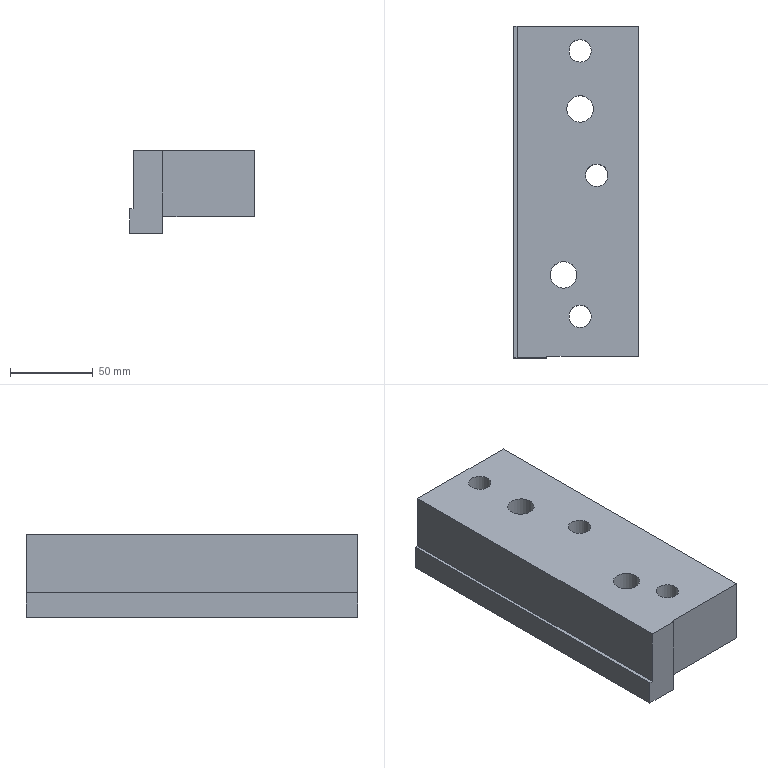Part | NX | features solid 2 | 1 solid | 22 faces | box 75 x 200 x 50 mm | volume 583540 mm3 | plane 14 | cylinder 8 | commonest cylinder face diameters 13.5 x3 19.5 x3 16 x2
STEP:
#1=CARTESIAN_POINT('',(1320.,131.,3.));
#2=VERTEX_POINT('',#1);
#3=CARTESIAN_POINT('',(1320.,131.,43.));
#4=VERTEX_POINT('',#3);
#5=CARTESIAN_POINT('',(1320.,131.,-7.));
#6=DIRECTION('',(0.,0.,1.));
#7=VECTOR('',#6,1000.);
#8=LINE('',#5,#7);
#9=EDGE_CURVE('',#2,#4,#8,.T.);
#10=ORIENTED_EDGE('',*,*,#9,.F.);
#11=CARTESIAN_POINT('',(1320.,330.,3.));
#12=VERTEX_POINT('',#11);
#13=CARTESIAN_POINT('',(1320.,330.,3.));
#14=DIRECTION('',(0.,-1.,0.));
#15=VECTOR('',#14,1000.);
#16=LINE('',#13,#15);
#17=EDGE_CURVE('',#12,#2,#16,.T.);
#18=ORIENTED_EDGE('',*,*,#17,.F.);
#19=CARTESIAN_POINT('',(1320.,330.,43.));
#20=VERTEX_POINT('',#19);
#21=CARTESIAN_POINT('',(1320.,330.,-7.));
#22=DIRECTION('',(0.,0.,-1.));
#23=VECTOR('',#22,1000.);
#24=LINE('',#21,#23);
#25=EDGE_CURVE('',#20,#12,#24,.T.);
#26=ORIENTED_EDGE('',*,*,#25,.F.);
#27=CARTESIAN_POINT('',(1320.,330.,43.));
#28=DIRECTION('',(0.,-1.,0.));
#29=VECTOR('',#28,1000.);
#30=LINE('',#27,#29);
#31=EDGE_CURVE('',#20,#4,#30,.T.);
#32=ORIENTED_EDGE('',*,*,#31,.T.);
#33=EDGE_LOOP('',(#10,#18,#26,#32));
#34=FACE_BOUND('',#33,.T.);
#35=CARTESIAN_POINT('',(1320.,330.,-7.));
#36=DIRECTION('',(-1.,0.,0.));
#37=DIRECTION('',(0.,0.,1.));
#38=AXIS2_PLACEMENT_3D('',#35,#36,#37);
#39=PLANE('',#38);
#40=ADVANCED_FACE('',(#34),#39,.F.);
#41=CARTESIAN_POINT('',(1247.,130.,43.));
#42=VERTEX_POINT('',#41);
#43=CARTESIAN_POINT('',(1265.,130.,43.));
#44=VERTEX_POINT('',#43);
#45=CARTESIAN_POINT('',(1245.,130.,43.));
#46=DIRECTION('',(1.,0.,0.));
#47=VECTOR('',#46,1000.);
#48=LINE('',#45,#47);
#49=EDGE_CURVE('',#42,#44,#48,.T.);
#50=ORIENTED_EDGE('',*,*,#49,.T.);
#51=CARTESIAN_POINT('',(1265.,131.,43.));
#52=VERTEX_POINT('',#51);
#53=CARTESIAN_POINT('',(1265.,390.,43.));
#54=DIRECTION('',(0.,1.,0.));
#55=VECTOR('',#54,1000.);
#56=LINE('',#53,#55);
#57=EDGE_CURVE('',#52,#44,#56,.F.);
#58=ORIENTED_EDGE('',*,*,#57,.F.);
#59=CARTESIAN_POINT('',(1319.,131.,43.));
#60=DIRECTION('',(1.,0.,0.));
#61=VECTOR('',#60,1000.);
#62=LINE('',#59,#61);
#63=EDGE_CURVE('',#52,#4,#62,.T.);
#64=ORIENTED_EDGE('',*,*,#63,.T.);
#65=ORIENTED_EDGE('',*,*,#31,.F.);
#66=CARTESIAN_POINT('',(1247.,330.,43.));
#67=VERTEX_POINT('',#66);
#68=CARTESIAN_POINT('',(1245.,330.,43.));
#69=DIRECTION('',(1.,0.,0.));
#70=VECTOR('',#69,1000.);
#71=LINE('',#68,#70);
#72=EDGE_CURVE('',#67,#20,#71,.T.);
#73=ORIENTED_EDGE('',*,*,#72,.F.);
#74=CARTESIAN_POINT('',(1247.,390.,43.));
#75=DIRECTION('',(0.,1.,0.));
#76=VECTOR('',#75,1000.);
#77=LINE('',#74,#76);
#78=EDGE_CURVE('',#67,#42,#77,.F.);
#79=ORIENTED_EDGE('',*,*,#78,.T.);
#80=EDGE_LOOP('',(#50,#58,#64,#65,#73,#79));
#81=FACE_BOUND('',#80,.T.);
#82=CARTESIAN_POINT('',(1275.,172.,43.));
#83=VERTEX_POINT('',#82);
#84=CARTESIAN_POINT('',(1275.,180.,43.));
#85=DIRECTION('',(0.,0.,1.));
#86=DIRECTION('',(0.,-1.,0.));
#87=AXIS2_PLACEMENT_3D('',#84,#85,#86);
#88=CIRCLE('',#87,8.);
#89=EDGE_CURVE('',#83,#83,#88,.T.);
#90=ORIENTED_EDGE('',*,*,#89,.F.);
#91=EDGE_LOOP('',(#90));
#92=FACE_BOUND('',#91,.T.);
#93=CARTESIAN_POINT('',(1285.,148.25,43.));
#94=VERTEX_POINT('',#93);
#95=CARTESIAN_POINT('',(1285.,155.,43.));
#96=DIRECTION('',(0.,0.,1.));
#97=DIRECTION('',(0.,-1.,0.));
#98=AXIS2_PLACEMENT_3D('',#95,#96,#97);
#99=CIRCLE('',#98,6.75);
#100=EDGE_CURVE('',#94,#94,#99,.T.);
#101=ORIENTED_EDGE('',*,*,#100,.F.);
#102=EDGE_LOOP('',(#101));
#103=FACE_BOUND('',#102,.T.);
#104=CARTESIAN_POINT('',(1295.,233.25,43.));
#105=VERTEX_POINT('',#104);
#106=CARTESIAN_POINT('',(1295.,240.,43.));
#107=DIRECTION('',(0.,0.,1.));
#108=DIRECTION('',(0.,-1.,0.));
#109=AXIS2_PLACEMENT_3D('',#106,#107,#108);
#110=CIRCLE('',#109,6.75);
#111=EDGE_CURVE('',#105,#105,#110,.T.);
#112=ORIENTED_EDGE('',*,*,#111,.F.);
#113=EDGE_LOOP('',(#112));
#114=FACE_BOUND('',#113,.T.);
#115=CARTESIAN_POINT('',(1285.,308.25,43.));
#116=VERTEX_POINT('',#115);
#117=CARTESIAN_POINT('',(1285.,315.,43.));
#118=DIRECTION('',(0.,0.,1.));
#119=DIRECTION('',(0.,-1.,0.));
#120=AXIS2_PLACEMENT_3D('',#117,#118,#119);
#121=CIRCLE('',#120,6.75);
#122=EDGE_CURVE('',#116,#116,#121,.T.);
#123=ORIENTED_EDGE('',*,*,#122,.F.);
#124=EDGE_LOOP('',(#123));
#125=FACE_BOUND('',#124,.T.);
#126=CARTESIAN_POINT('',(1285.,288.,43.));
#127=VERTEX_POINT('',#126);
#128=CARTESIAN_POINT('',(1285.,280.,43.));
#129=DIRECTION('',(0.,0.,-1.));
#130=DIRECTION('',(0.,1.,0.));
#131=AXIS2_PLACEMENT_3D('',#128,#129,#130);
#132=CIRCLE('',#131,8.);
#133=EDGE_CURVE('',#127,#127,#132,.F.);
#134=ORIENTED_EDGE('',*,*,#133,.F.);
#135=EDGE_LOOP('',(#134));
#136=FACE_BOUND('',#135,.T.);
#137=CARTESIAN_POINT('',(1245.,390.,43.));
#138=DIRECTION('',(0.,0.,-1.));
#139=DIRECTION('',(0.,-1.,0.));
#140=AXIS2_PLACEMENT_3D('',#137,#138,#139);
#141=PLANE('',#140);
#142=ADVANCED_FACE('',(#81,#92,#103,#114,#125,#136),#141,.F.);
#143=CARTESIAN_POINT('',(1265.,131.,3.));
#144=VERTEX_POINT('',#143);
#145=CARTESIAN_POINT('',(1319.,131.,3.));
#146=DIRECTION('',(1.,0.,0.));
#147=VECTOR('',#146,1000.);
#148=LINE('',#145,#147);
#149=EDGE_CURVE('',#144,#2,#148,.T.);
#150=ORIENTED_EDGE('',*,*,#149,.F.);
#151=CARTESIAN_POINT('',(1265.,330.,3.));
#152=VERTEX_POINT('',#151);
#153=CARTESIAN_POINT('',(1265.,415.,3.));
#154=DIRECTION('',(0.,-1.,0.));
#155=VECTOR('',#154,1000.);
#156=LINE('',#153,#155);
#157=EDGE_CURVE('',#152,#144,#156,.T.);
#158=ORIENTED_EDGE('',*,*,#157,.F.);
#159=CARTESIAN_POINT('',(1265.,330.,3.));
#160=DIRECTION('',(1.,0.,0.));
#161=VECTOR('',#160,1000.);
#162=LINE('',#159,#161);
#163=EDGE_CURVE('',#152,#12,#162,.T.);
#164=ORIENTED_EDGE('',*,*,#163,.T.);
#165=ORIENTED_EDGE('',*,*,#17,.T.);
#166=EDGE_LOOP('',(#150,#158,#164,#165));
#167=FACE_BOUND('',#166,.T.);
#168=CARTESIAN_POINT('',(1295.,249.75,3.));
#169=VERTEX_POINT('',#168);
#170=CARTESIAN_POINT('',(1295.,240.,3.));
#171=DIRECTION('',(0.,0.,-1.));
#172=DIRECTION('',(0.,1.,0.));
#173=AXIS2_PLACEMENT_3D('',#170,#171,#172);
#174=CIRCLE('',#173,9.75);
#175=EDGE_CURVE('',#169,#169,#174,.F.);
#176=ORIENTED_EDGE('',*,*,#175,.T.);
#177=EDGE_LOOP('',(#176));
#178=FACE_BOUND('',#177,.T.);
#179=CARTESIAN_POINT('',(1275.,188.,3.));
#180=VERTEX_POINT('',#179);
#181=CARTESIAN_POINT('',(1275.,180.,3.));
#182=DIRECTION('',(0.,0.,-1.));
#183=DIRECTION('',(0.,1.,0.));
#184=AXIS2_PLACEMENT_3D('',#181,#182,#183);
#185=CIRCLE('',#184,8.);
#186=EDGE_CURVE('',#180,#180,#185,.F.);
#187=ORIENTED_EDGE('',*,*,#186,.T.);
#188=EDGE_LOOP('',(#187));
#189=FACE_BOUND('',#188,.T.);
#190=CARTESIAN_POINT('',(1285.,164.75,3.));
#191=VERTEX_POINT('',#190);
#192=CARTESIAN_POINT('',(1285.,155.,3.));
#193=DIRECTION('',(0.,0.,-1.));
#194=DIRECTION('',(0.,1.,0.));
#195=AXIS2_PLACEMENT_3D('',#192,#193,#194);
#196=CIRCLE('',#195,9.75);
#197=EDGE_CURVE('',#191,#191,#196,.F.);
#198=ORIENTED_EDGE('',*,*,#197,.T.);
#199=EDGE_LOOP('',(#198));
#200=FACE_BOUND('',#199,.T.);
#201=CARTESIAN_POINT('',(1285.,324.75,3.));
#202=VERTEX_POINT('',#201);
#203=CARTESIAN_POINT('',(1285.,315.,3.));
#204=DIRECTION('',(0.,0.,-1.));
#205=DIRECTION('',(0.,1.,0.));
#206=AXIS2_PLACEMENT_3D('',#203,#204,#205);
#207=CIRCLE('',#206,9.75);
#208=EDGE_CURVE('',#202,#202,#207,.F.);
#209=ORIENTED_EDGE('',*,*,#208,.T.);
#210=EDGE_LOOP('',(#209));
#211=FACE_BOUND('',#210,.T.);
#212=CARTESIAN_POINT('',(1285.,288.,3.));
#213=VERTEX_POINT('',#212);
#214=CARTESIAN_POINT('',(1285.,280.,3.));
#215=DIRECTION('',(0.,0.,-1.));
#216=DIRECTION('',(0.,1.,0.));
#217=AXIS2_PLACEMENT_3D('',#214,#215,#216);
#218=CIRCLE('',#217,8.);
#219=EDGE_CURVE('',#213,#213,#218,.F.);
#220=ORIENTED_EDGE('',*,*,#219,.T.);
#221=EDGE_LOOP('',(#220));
#222=FACE_BOUND('',#221,.T.);
#223=CARTESIAN_POINT('',(1265.,415.,3.));
#224=DIRECTION('',(0.,0.,-1.));
#225=DIRECTION('',(0.,-1.,0.));
#226=AXIS2_PLACEMENT_3D('',#223,#224,#225);
#227=PLANE('',#226);
#228=ADVANCED_FACE('',(#167,#178,#189,#200,#211,#222),#227,.T.);
#229=CARTESIAN_POINT('',(1247.,330.,8.));
#230=VERTEX_POINT('',#229);
#231=CARTESIAN_POINT('',(1247.,330.,43.));
#232=DIRECTION('',(0.,0.,1.));
#233=VECTOR('',#232,1000.);
#234=LINE('',#231,#233);
#235=EDGE_CURVE('',#230,#67,#234,.T.);
#236=ORIENTED_EDGE('',*,*,#235,.T.);
#237=ORIENTED_EDGE('',*,*,#72,.T.);
#238=ORIENTED_EDGE('',*,*,#25,.T.);
#239=ORIENTED_EDGE('',*,*,#163,.F.);
#240=CARTESIAN_POINT('',(1265.,330.,-7.));
#241=VERTEX_POINT('',#240);
#242=CARTESIAN_POINT('',(1265.,330.,-7.));
#243=DIRECTION('',(0.,0.,-1.));
#244=VECTOR('',#243,1000.);
#245=LINE('',#242,#244);
#246=EDGE_CURVE('',#152,#241,#245,.T.);
#247=ORIENTED_EDGE('',*,*,#246,.T.);
#248=CARTESIAN_POINT('',(1245.,330.,-7.));
#249=VERTEX_POINT('',#248);
#250=CARTESIAN_POINT('',(1245.,330.,-7.));
#251=DIRECTION('',(1.,0.,0.));
#252=VECTOR('',#251,1000.);
#253=LINE('',#250,#252);
#254=EDGE_CURVE('',#241,#249,#253,.F.);
#255=ORIENTED_EDGE('',*,*,#254,.T.);
#256=CARTESIAN_POINT('',(1245.,330.,8.));
#257=VERTEX_POINT('',#256);
#258=CARTESIAN_POINT('',(1245.,330.,-7.));
#259=DIRECTION('',(0.,0.,-1.));
#260=VECTOR('',#259,1000.);
#261=LINE('',#258,#260);
#262=EDGE_CURVE('',#257,#249,#261,.T.);
#263=ORIENTED_EDGE('',*,*,#262,.F.);
#264=CARTESIAN_POINT('',(1245.,330.,8.));
#265=DIRECTION('',(-1.,0.,0.));
#266=VECTOR('',#265,1000.);
#267=LINE('',#264,#266);
#268=EDGE_CURVE('',#257,#230,#267,.F.);
#269=ORIENTED_EDGE('',*,*,#268,.T.);
#270=EDGE_LOOP('',(#236,#237,#238,#239,#247,#255,#263,#269));
#271=FACE_BOUND('',#270,.T.);
#272=CARTESIAN_POINT('',(1245.,330.,8.));
#273=DIRECTION('',(0.,1.,0.));
#274=DIRECTION('',(0.,0.,1.));
#275=AXIS2_PLACEMENT_3D('',#272,#273,#274);
#276=PLANE('',#275);
#277=ADVANCED_FACE('',(#271),#276,.T.);
#278=CARTESIAN_POINT('',(1295.,233.25,18.));
#279=VERTEX_POINT('',#278);
#280=CARTESIAN_POINT('',(1295.,240.,18.));
#281=DIRECTION('',(0.,0.,1.));
#282=DIRECTION('',(0.,-1.,0.));
#283=AXIS2_PLACEMENT_3D('',#280,#281,#282);
#284=CIRCLE('',#283,6.75);
#285=EDGE_CURVE('',#279,#279,#284,.T.);
#286=ORIENTED_EDGE('',*,*,#285,.T.);
#287=EDGE_LOOP('',(#286));
#288=FACE_BOUND('',#287,.T.);
#289=CARTESIAN_POINT('',(1295.,230.25,18.));
#290=VERTEX_POINT('',#289);
#291=CARTESIAN_POINT('',(1295.,240.,18.));
#292=DIRECTION('',(0.,0.,1.));
#293=DIRECTION('',(0.,-1.,0.));
#294=AXIS2_PLACEMENT_3D('',#291,#292,#293);
#295=CIRCLE('',#294,9.75);
#296=EDGE_CURVE('',#290,#290,#295,.T.);
#297=ORIENTED_EDGE('',*,*,#296,.F.);
#298=EDGE_LOOP('',(#297));
#299=FACE_BOUND('',#298,.T.);
#300=CARTESIAN_POINT('',(1295.,240.,18.));
#301=DIRECTION('',(0.,0.,1.));
#302=DIRECTION('',(0.,-1.,0.));
#303=AXIS2_PLACEMENT_3D('',#300,#301,#302);
#304=PLANE('',#303);
#305=ADVANCED_FACE('',(#288,#299),#304,.F.);
#306=CARTESIAN_POINT('',(1285.,148.25,18.));
#307=VERTEX_POINT('',#306);
#308=CARTESIAN_POINT('',(1285.,155.,18.));
#309=DIRECTION('',(0.,0.,1.));
#310=DIRECTION('',(0.,-1.,0.));
#311=AXIS2_PLACEMENT_3D('',#308,#309,#310);
#312=CIRCLE('',#311,6.75);
#313=EDGE_CURVE('',#307,#307,#312,.T.);
#314=ORIENTED_EDGE('',*,*,#313,.T.);
#315=EDGE_LOOP('',(#314));
#316=FACE_BOUND('',#315,.T.);
#317=CARTESIAN_POINT('',(1285.,145.25,18.));
#318=VERTEX_POINT('',#317);
#319=CARTESIAN_POINT('',(1285.,155.,18.));
#320=DIRECTION('',(0.,0.,1.));
#321=DIRECTION('',(0.,-1.,0.));
#322=AXIS2_PLACEMENT_3D('',#319,#320,#321);
#323=CIRCLE('',#322,9.75);
#324=EDGE_CURVE('',#318,#318,#323,.T.);
#325=ORIENTED_EDGE('',*,*,#324,.F.);
#326=EDGE_LOOP('',(#325));
#327=FACE_BOUND('',#326,.T.);
#328=CARTESIAN_POINT('',(1285.,155.,18.));
#329=DIRECTION('',(0.,0.,1.));
#330=DIRECTION('',(0.,-1.,0.));
#331=AXIS2_PLACEMENT_3D('',#328,#329,#330);
#332=PLANE('',#331);
#333=ADVANCED_FACE('',(#316,#327),#332,.F.);
#334=CARTESIAN_POINT('',(1285.,308.25,18.));
#335=VERTEX_POINT('',#334);
#336=CARTESIAN_POINT('',(1285.,315.,18.));
#337=DIRECTION('',(0.,0.,1.));
#338=DIRECTION('',(0.,-1.,0.));
#339=AXIS2_PLACEMENT_3D('',#336,#337,#338);
#340=CIRCLE('',#339,6.75);
#341=EDGE_CURVE('',#335,#335,#340,.T.);
#342=ORIENTED_EDGE('',*,*,#341,.T.);
#343=EDGE_LOOP('',(#342));
#344=FACE_BOUND('',#343,.T.);
#345=CARTESIAN_POINT('',(1285.,305.25,18.));
#346=VERTEX_POINT('',#345);
#347=CARTESIAN_POINT('',(1285.,315.,18.));
#348=DIRECTION('',(0.,0.,1.));
#349=DIRECTION('',(0.,-1.,0.));
#350=AXIS2_PLACEMENT_3D('',#347,#348,#349);
#351=CIRCLE('',#350,9.75);
#352=EDGE_CURVE('',#346,#346,#351,.T.);
#353=ORIENTED_EDGE('',*,*,#352,.F.);
#354=EDGE_LOOP('',(#353));
#355=FACE_BOUND('',#354,.T.);
#356=CARTESIAN_POINT('',(1285.,315.,18.));
#357=DIRECTION('',(0.,0.,1.));
#358=DIRECTION('',(0.,-1.,0.));
#359=AXIS2_PLACEMENT_3D('',#356,#357,#358);
#360=PLANE('',#359);
#361=ADVANCED_FACE('',(#344,#355),#360,.F.);
#362=ORIENTED_EDGE('',*,*,#100,.T.);
#363=EDGE_LOOP('',(#362));
#364=FACE_BOUND('',#363,.T.);
#365=ORIENTED_EDGE('',*,*,#313,.F.);
#366=EDGE_LOOP('',(#365));
#367=FACE_BOUND('',#366,.T.);
#368=CARTESIAN_POINT('',(1285.,155.,43.));
#369=DIRECTION('',(0.,0.,1.));
#370=DIRECTION('',(0.,-1.,0.));
#371=AXIS2_PLACEMENT_3D('',#368,#369,#370);
#372=CYLINDRICAL_SURFACE('',#371,6.75);
#373=ADVANCED_FACE('',(#364,#367),#372,.F.);
#374=ORIENTED_EDGE('',*,*,#111,.T.);
#375=EDGE_LOOP('',(#374));
#376=FACE_BOUND('',#375,.T.);
#377=ORIENTED_EDGE('',*,*,#285,.F.);
#378=EDGE_LOOP('',(#377));
#379=FACE_BOUND('',#378,.T.);
#380=CARTESIAN_POINT('',(1295.,240.,43.));
#381=DIRECTION('',(0.,0.,1.));
#382=DIRECTION('',(0.,-1.,0.));
#383=AXIS2_PLACEMENT_3D('',#380,#381,#382);
#384=CYLINDRICAL_SURFACE('',#383,6.75);
#385=ADVANCED_FACE('',(#376,#379),#384,.F.);
#386=ORIENTED_EDGE('',*,*,#122,.T.);
#387=EDGE_LOOP('',(#386));
#388=FACE_BOUND('',#387,.T.);
#389=ORIENTED_EDGE('',*,*,#341,.F.);
#390=EDGE_LOOP('',(#389));
#391=FACE_BOUND('',#390,.T.);
#392=CARTESIAN_POINT('',(1285.,315.,43.));
#393=DIRECTION('',(0.,0.,1.));
#394=DIRECTION('',(0.,-1.,0.));
#395=AXIS2_PLACEMENT_3D('',#392,#393,#394);
#396=CYLINDRICAL_SURFACE('',#395,6.75);
#397=ADVANCED_FACE('',(#388,#391),#396,.F.);
#398=ORIENTED_EDGE('',*,*,#296,.T.);
#399=EDGE_LOOP('',(#398));
#400=FACE_BOUND('',#399,.T.);
#401=ORIENTED_EDGE('',*,*,#175,.F.);
#402=EDGE_LOOP('',(#401));
#403=FACE_BOUND('',#402,.T.);
#404=CARTESIAN_POINT('',(1295.,240.,-7.));
#405=DIRECTION('',(0.,0.,1.));
#406=DIRECTION('',(0.,-1.,0.));
#407=AXIS2_PLACEMENT_3D('',#404,#405,#406);
#408=CYLINDRICAL_SURFACE('',#407,9.75);
#409=ADVANCED_FACE('',(#400,#403),#408,.F.);
#410=ORIENTED_EDGE('',*,*,#89,.T.);
#411=EDGE_LOOP('',(#410));
#412=FACE_BOUND('',#411,.T.);
#413=ORIENTED_EDGE('',*,*,#186,.F.);
#414=EDGE_LOOP('',(#413));
#415=FACE_BOUND('',#414,.T.);
#416=CARTESIAN_POINT('',(1275.,180.,-7.));
#417=DIRECTION('',(0.,0.,1.));
#418=DIRECTION('',(0.,-1.,0.));
#419=AXIS2_PLACEMENT_3D('',#416,#417,#418);
#420=CYLINDRICAL_SURFACE('',#419,8.);
#421=ADVANCED_FACE('',(#412,#415),#420,.F.);
#422=ORIENTED_EDGE('',*,*,#324,.T.);
#423=EDGE_LOOP('',(#422));
#424=FACE_BOUND('',#423,.T.);
#425=ORIENTED_EDGE('',*,*,#197,.F.);
#426=EDGE_LOOP('',(#425));
#427=FACE_BOUND('',#426,.T.);
#428=CARTESIAN_POINT('',(1285.,155.,-7.));
#429=DIRECTION('',(0.,0.,1.));
#430=DIRECTION('',(0.,-1.,0.));
#431=AXIS2_PLACEMENT_3D('',#428,#429,#430);
#432=CYLINDRICAL_SURFACE('',#431,9.75);
#433=ADVANCED_FACE('',(#424,#427),#432,.F.);
#434=ORIENTED_EDGE('',*,*,#352,.T.);
#435=EDGE_LOOP('',(#434));
#436=FACE_BOUND('',#435,.T.);
#437=ORIENTED_EDGE('',*,*,#208,.F.);
#438=EDGE_LOOP('',(#437));
#439=FACE_BOUND('',#438,.T.);
#440=CARTESIAN_POINT('',(1285.,315.,-7.));
#441=DIRECTION('',(0.,0.,1.));
#442=DIRECTION('',(0.,-1.,0.));
#443=AXIS2_PLACEMENT_3D('',#440,#441,#442);
#444=CYLINDRICAL_SURFACE('',#443,9.75);
#445=ADVANCED_FACE('',(#436,#439),#444,.F.);
#446=CARTESIAN_POINT('',(1265.,130.,-7.));
#447=VERTEX_POINT('',#446);
#448=CARTESIAN_POINT('',(1265.,130.,-7.));
#449=DIRECTION('',(0.,0.,1.));
#450=VECTOR('',#449,1000.);
#451=LINE('',#448,#450);
#452=EDGE_CURVE('',#447,#44,#451,.T.);
#453=ORIENTED_EDGE('',*,*,#452,.T.);
#454=ORIENTED_EDGE('',*,*,#49,.F.);
#455=CARTESIAN_POINT('',(1247.,130.,8.));
#456=VERTEX_POINT('',#455);
#457=CARTESIAN_POINT('',(1247.,130.,43.));
#458=DIRECTION('',(0.,0.,1.));
#459=VECTOR('',#458,1000.);
#460=LINE('',#457,#459);
#461=EDGE_CURVE('',#456,#42,#460,.T.);
#462=ORIENTED_EDGE('',*,*,#461,.F.);
#463=CARTESIAN_POINT('',(1245.,130.,8.));
#464=VERTEX_POINT('',#463);
#465=CARTESIAN_POINT('',(1245.,130.,8.));
#466=DIRECTION('',(-1.,0.,0.));
#467=VECTOR('',#466,1000.);
#468=LINE('',#465,#467);
#469=EDGE_CURVE('',#464,#456,#468,.F.);
#470=ORIENTED_EDGE('',*,*,#469,.F.);
#471=CARTESIAN_POINT('',(1245.,130.,-7.));
#472=VERTEX_POINT('',#471);
#473=CARTESIAN_POINT('',(1245.,130.,-7.));
#474=DIRECTION('',(0.,0.,-1.));
#475=VECTOR('',#474,1000.);
#476=LINE('',#473,#475);
#477=EDGE_CURVE('',#464,#472,#476,.T.);
#478=ORIENTED_EDGE('',*,*,#477,.T.);
#479=CARTESIAN_POINT('',(1245.,130.,-7.));
#480=DIRECTION('',(1.,0.,0.));
#481=VECTOR('',#480,1000.);
#482=LINE('',#479,#481);
#483=EDGE_CURVE('',#447,#472,#482,.F.);
#484=ORIENTED_EDGE('',*,*,#483,.F.);
#485=EDGE_LOOP('',(#453,#454,#462,#470,#478,#484));
#486=FACE_BOUND('',#485,.T.);
#487=CARTESIAN_POINT('',(1305.,130.,-7.));
#488=DIRECTION('',(0.,1.,0.));
#489=DIRECTION('',(0.,0.,1.));
#490=AXIS2_PLACEMENT_3D('',#487,#488,#489);
#491=PLANE('',#490);
#492=ADVANCED_FACE('',(#486),#491,.F.);
#493=ORIENTED_EDGE('',*,*,#246,.F.);
#494=ORIENTED_EDGE('',*,*,#157,.T.);
#495=CARTESIAN_POINT('',(1265.,131.,-7.));
#496=DIRECTION('',(0.,0.,1.));
#497=VECTOR('',#496,1000.);
#498=LINE('',#495,#497);
#499=EDGE_CURVE('',#52,#144,#498,.F.);
#500=ORIENTED_EDGE('',*,*,#499,.F.);
#501=ORIENTED_EDGE('',*,*,#57,.T.);
#502=ORIENTED_EDGE('',*,*,#452,.F.);
#503=CARTESIAN_POINT('',(1265.,330.,-7.));
#504=DIRECTION('',(0.,1.,0.));
#505=VECTOR('',#504,1000.);
#506=LINE('',#503,#505);
#507=EDGE_CURVE('',#241,#447,#506,.F.);
#508=ORIENTED_EDGE('',*,*,#507,.F.);
#509=EDGE_LOOP('',(#493,#494,#500,#501,#502,#508));
#510=FACE_BOUND('',#509,.T.);
#511=CARTESIAN_POINT('',(1265.,415.,-7.));
#512=DIRECTION('',(-1.,0.,0.));
#513=DIRECTION('',(0.,0.,1.));
#514=AXIS2_PLACEMENT_3D('',#511,#512,#513);
#515=PLANE('',#514);
#516=ADVANCED_FACE('',(#510),#515,.F.);
#517=ORIENTED_EDGE('',*,*,#254,.F.);
#518=ORIENTED_EDGE('',*,*,#507,.T.);
#519=ORIENTED_EDGE('',*,*,#483,.T.);
#520=CARTESIAN_POINT('',(1245.,330.,-7.));
#521=DIRECTION('',(0.,1.,0.));
#522=VECTOR('',#521,1000.);
#523=LINE('',#520,#522);
#524=EDGE_CURVE('',#249,#472,#523,.F.);
#525=ORIENTED_EDGE('',*,*,#524,.F.);
#526=EDGE_LOOP('',(#517,#518,#519,#525));
#527=FACE_BOUND('',#526,.T.);
#528=CARTESIAN_POINT('',(1245.,330.,-7.));
#529=DIRECTION('',(0.,0.,-1.));
#530=DIRECTION('',(0.,-1.,0.));
#531=AXIS2_PLACEMENT_3D('',#528,#529,#530);
#532=PLANE('',#531);
#533=ADVANCED_FACE('',(#527),#532,.T.);
#534=CARTESIAN_POINT('',(1245.,390.,8.));
#535=DIRECTION('',(0.,-1.,0.));
#536=VECTOR('',#535,1000.);
#537=LINE('',#534,#536);
#538=EDGE_CURVE('',#257,#464,#537,.T.);
#539=ORIENTED_EDGE('',*,*,#538,.F.);
#540=ORIENTED_EDGE('',*,*,#262,.T.);
#541=ORIENTED_EDGE('',*,*,#524,.T.);
#542=ORIENTED_EDGE('',*,*,#477,.F.);
#543=EDGE_LOOP('',(#539,#540,#541,#542));
#544=FACE_BOUND('',#543,.T.);
#545=CARTESIAN_POINT('',(1245.,390.,-7.));
#546=DIRECTION('',(-1.,0.,0.));
#547=DIRECTION('',(0.,0.,1.));
#548=AXIS2_PLACEMENT_3D('',#545,#546,#547);
#549=PLANE('',#548);
#550=ADVANCED_FACE('',(#544),#549,.T.);
#551=ORIENTED_EDGE('',*,*,#268,.F.);
#552=ORIENTED_EDGE('',*,*,#538,.T.);
#553=ORIENTED_EDGE('',*,*,#469,.T.);
#554=CARTESIAN_POINT('',(1247.,390.,8.));
#555=DIRECTION('',(0.,1.,0.));
#556=VECTOR('',#555,1000.);
#557=LINE('',#554,#556);
#558=EDGE_CURVE('',#230,#456,#557,.F.);
#559=ORIENTED_EDGE('',*,*,#558,.F.);
#560=EDGE_LOOP('',(#551,#552,#553,#559));
#561=FACE_BOUND('',#560,.T.);
#562=CARTESIAN_POINT('',(1245.,390.,8.));
#563=DIRECTION('',(0.,0.,1.));
#564=DIRECTION('',(0.,-1.,0.));
#565=AXIS2_PLACEMENT_3D('',#562,#563,#564);
#566=PLANE('',#565);
#567=ADVANCED_FACE('',(#561),#566,.T.);
#568=ORIENTED_EDGE('',*,*,#235,.F.);
#569=ORIENTED_EDGE('',*,*,#558,.T.);
#570=ORIENTED_EDGE('',*,*,#461,.T.);
#571=ORIENTED_EDGE('',*,*,#78,.F.);
#572=EDGE_LOOP('',(#568,#569,#570,#571));
#573=FACE_BOUND('',#572,.T.);
#574=CARTESIAN_POINT('',(1247.,390.,43.));
#575=DIRECTION('',(1.,0.,0.));
#576=DIRECTION('',(0.,0.,-1.));
#577=AXIS2_PLACEMENT_3D('',#574,#575,#576);
#578=PLANE('',#577);
#579=ADVANCED_FACE('',(#573),#578,.F.);
#580=ORIENTED_EDGE('',*,*,#219,.F.);
#581=EDGE_LOOP('',(#580));
#582=FACE_BOUND('',#581,.T.);
#583=ORIENTED_EDGE('',*,*,#133,.T.);
#584=EDGE_LOOP('',(#583));
#585=FACE_BOUND('',#584,.T.);
#586=CARTESIAN_POINT('',(1285.,280.,103.));
#587=DIRECTION('',(0.,0.,-1.));
#588=DIRECTION('',(-1.,0.,0.));
#589=AXIS2_PLACEMENT_3D('',#586,#587,#588);
#590=CYLINDRICAL_SURFACE('',#589,8.);
#591=ADVANCED_FACE('',(#582,#585),#590,.F.);
#592=ORIENTED_EDGE('',*,*,#9,.T.);
#593=ORIENTED_EDGE('',*,*,#63,.F.);
#594=ORIENTED_EDGE('',*,*,#499,.T.);
#595=ORIENTED_EDGE('',*,*,#149,.T.);
#596=EDGE_LOOP('',(#592,#593,#594,#595));
#597=FACE_BOUND('',#596,.T.);
#598=CARTESIAN_POINT('',(1319.,131.,43.));
#599=DIRECTION('',(0.,-1.,0.));
#600=DIRECTION('',(0.,0.,-1.));
#601=AXIS2_PLACEMENT_3D('',#598,#599,#600);
#602=PLANE('',#601);
#603=ADVANCED_FACE('',(#597),#602,.T.);
#604=CLOSED_SHELL('',(#40,#142,#228,#277,#305,#333,#361,#373,#385,#397,#409,#421,#433,#445,#492,#516,#533,#550,#567,#579,#591,#603));
#605=MANIFOLD_SOLID_BREP('',#604);
#606=(LENGTH_UNIT()NAMED_UNIT(*)SI_UNIT(.MILLI.,.METRE.));
#607=UNCERTAINTY_MEASURE_WITH_UNIT(LENGTH_MEASURE(0.00001),#606,'','');
#608=(NAMED_UNIT(*)PLANE_ANGLE_UNIT()SI_UNIT($,.RADIAN.));
#609=(NAMED_UNIT(*)SI_UNIT($,.STERADIAN.)SOLID_ANGLE_UNIT());
#610=(GEOMETRIC_REPRESENTATION_CONTEXT(3)GLOBAL_UNCERTAINTY_ASSIGNED_CONTEXT((#607))GLOBAL_UNIT_ASSIGNED_CONTEXT((#606,#608,#609))REPRESENTATION_CONTEXT('',''));
#611=ADVANCED_BREP_SHAPE_REPRESENTATION('',(#605),#610);